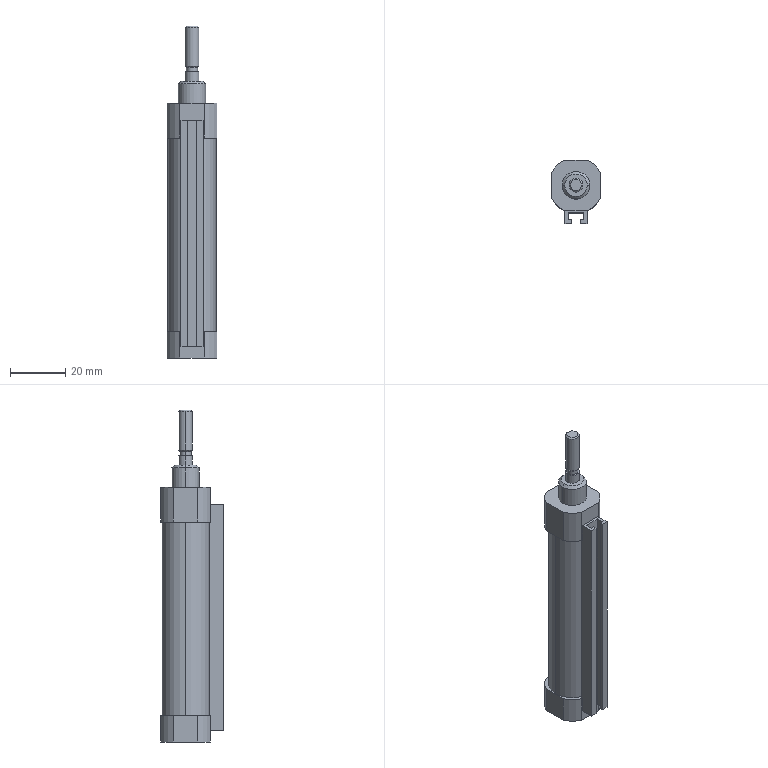Part | STEP file | CDJ2B16_45_B_0_ | 1 solid | 65 faces | box 18 x 22.7 x 120 mm | volume 25727 mm3 | plane 32 | cylinder 23 | cone 10 | commonest cylinder face diameters 20 x8 4.13 x4 5 x4 17.4 x3 4.02 x2 10 x2